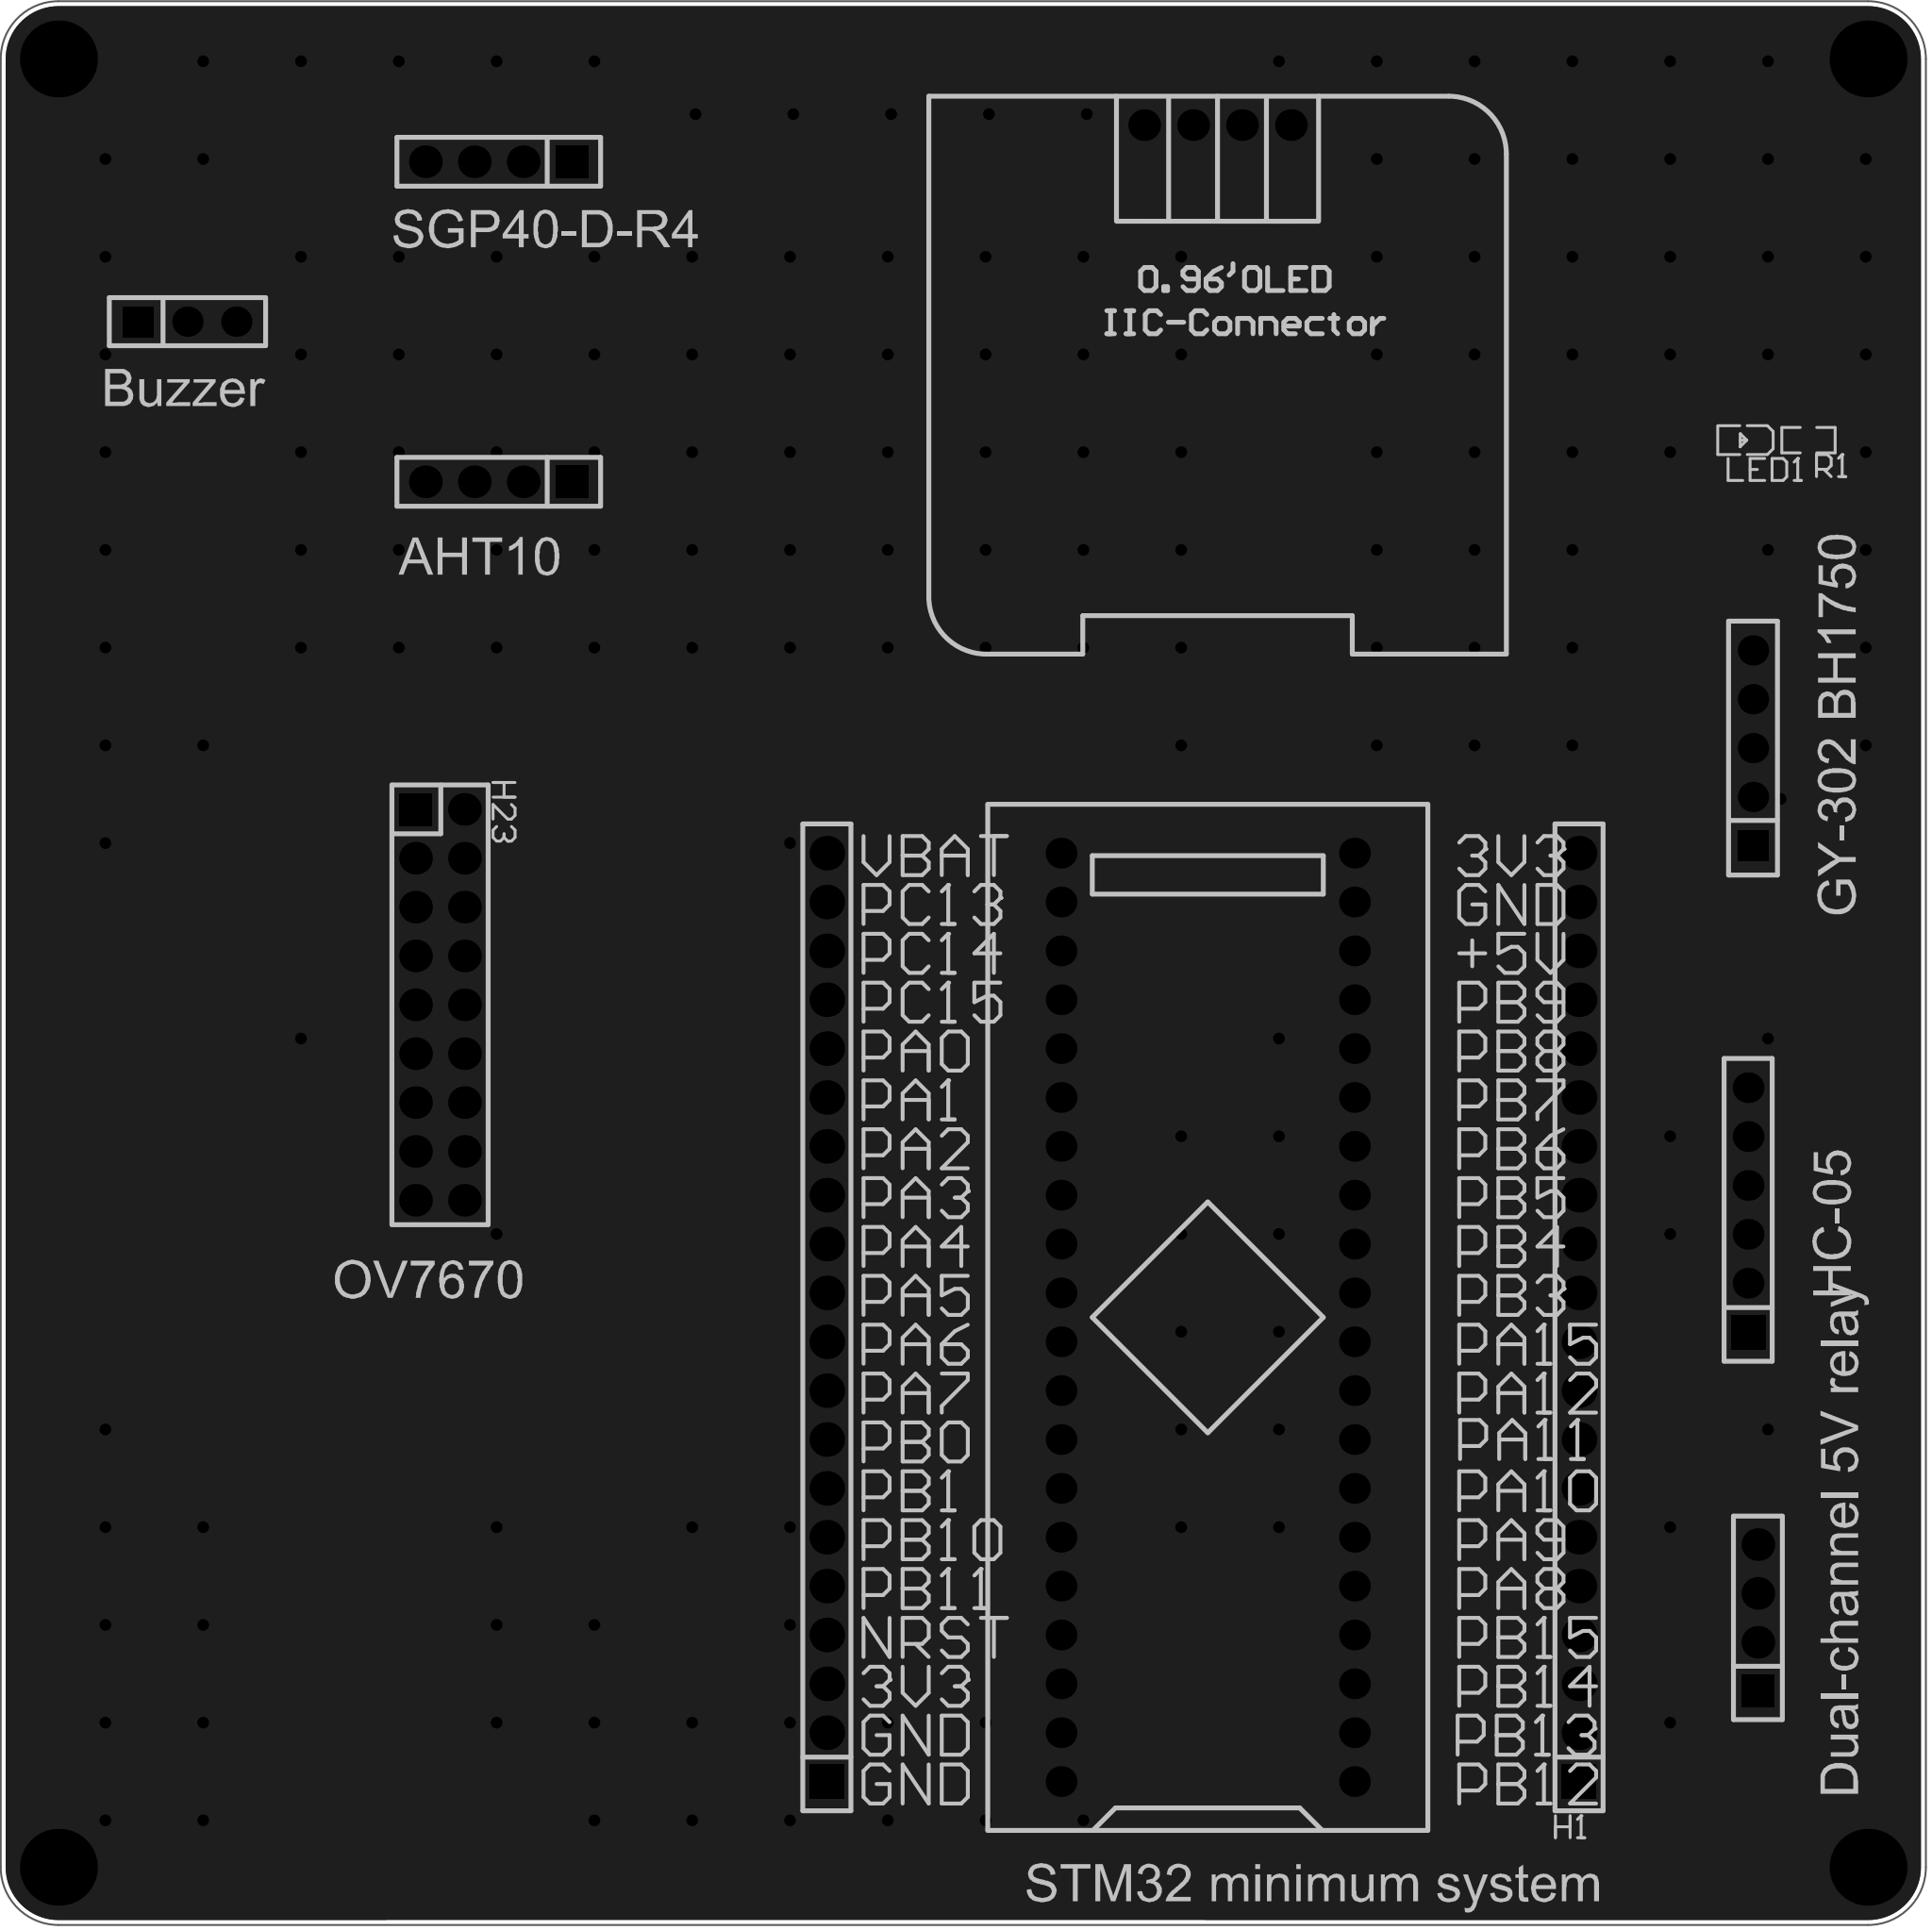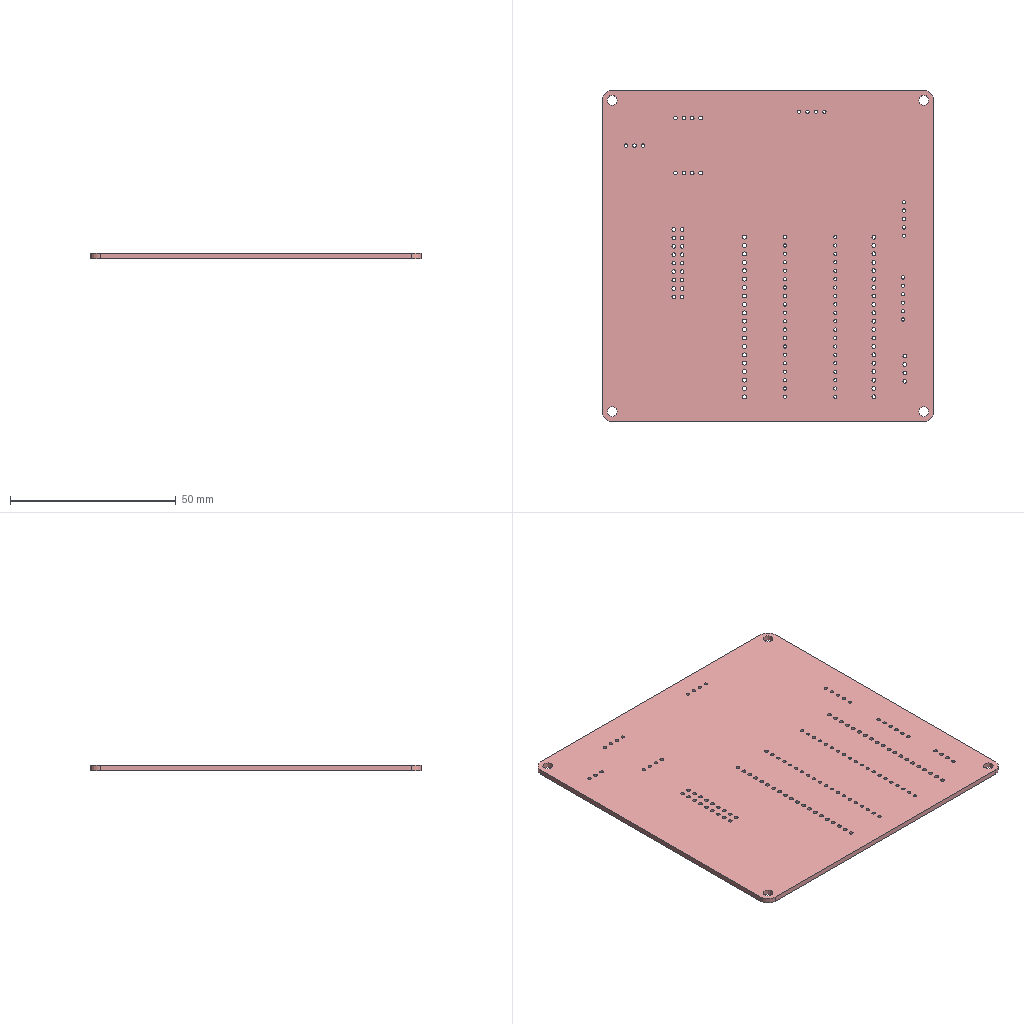Circuit board layout | Altium Designer | box 100 x 100 x 1.6 mm
Layer stack:
# Altium Designer layer stack of  (unit mm; dielectric type: 0 none, 1 core, 2 prepreg, 3 surface material)
index,name,kind,layer,copper_thickness_mm,dielectric_type,dielectric_thickness_mm,dielectric_material,dielectric_constant
0,Top Paste Mask Layer,other,,,,,,
1,Top Silkscreen Layer,other,,,,,,
2,Top Solder Mask Layer,dielectric,,,3,0.01,,3.3
3,Top Layer,copper,Top Layer,0.035,,,,
4,Dielectric1,dielectric,,,3,1.51,FR4,4.5
5,Bottom Layer,copper,Bottom Layer,0.035,,,,
6,Bottom Solder Mask Layer,dielectric,,,3,0.01,,3.3
7,Bottom Silkscreen Layer,other,,,,,,
8,Bottom Paste Mask Layer,other,,,,,,
# drill layer pairs: low layer,high layer
drill_pair,Top Layer,Bottom Layer
Part placement:
Designator,Comment,Layer,Footprint,Center-X(mm),Center-Y(mm),Rotation
U1,STM32F103C8T6-Card,TopLayer,CONN-TH_L53.3-W22.9_STM32F103C8T6-CARD,143.256,110.49,90
H23,,TopLayer,HDR-TH_18P-P2.54-V-M-R2-C9-S2.54,103.375,126.737,270
H19,,TopLayer,HDR-TH_4P-P2.54-V-F,106.426,153.924,180
OLED1,,TopLayer,0.96OLED_4P,143.764,172.466,0
H20,,TopLayer,HDR-TH_4P-P2.54-V-F,106.426,170.561,180
H21,,TopLayer,HDR-TH_5P-P2.54-V-F,171.577,140.081,90
H22,,TopLayer,HDR-TH_4P-P2.54-V-F,171.831,94.869,90
H1,,TopLayer,HDR-TH_20P-P2.54-V-F,162.539,110.49,90
H2,,TopLayer,HDR-TH_20P-P2.54-V-F,123.468,110.49,90
H25,,TopLayer,HDR-TH_3P-P2.54-V-F,90.256,162.248,0
LED1,,TopLayer,LED_0603,171.134,156.096,180
R1,510,TopLayer,R0603,174.458,156.088,0
H24,,TopLayer,HDR-TH_6P-P2.54-V-F,171.323,116.078,90
Pad and via stacks:
# Altium Designer via and pad stacks of  (unit mm). Each distinct definition once, with the count of objects using it.
# via: kind,start_layer,end_layer,hole_mm,diameter_mm,mode(0 simple;1 top-mid-bottom;2 full stack),diameter_per_layer,count,example_net
# pad: kind,layer,hole_mm,hole_type(0 round;1 square;2 slot),plating,top_size,top_shape(1 round;2 rect;3 octagon;9 rounded rect),mid_size,bottom_size,mode,footprint,size_per_layer,count,example
pad,Multi-Layer,3,0,plated,4x4,1,4x4,4x4,0,,,4,1
pad,Multi-Layer,1,0,plated,1.6x1.6,1,1.6x1.6,1.6x1.6,0,CONN-TH_L53.3-W22.9_STM32F103C8T6-CARD,,40,U1.1
pad,Multi-Layer,1.1,0,plated,1.7x1.7,2,1.7x1.7,1.7x1.7,0,HDR-TH_18P-P2.54-V-M-R2-C9-S2.54,,1,H23.1
pad,Multi-Layer,1.1,0,plated,1.7x1.7,1,1.7x1.7,1.7x1.7,0,HDR-TH_18P-P2.54-V-M-R2-C9-S2.54,,17,H23.2
pad,Multi-Layer,1.1,0,plated,1.7x1.7,2,1.7x1.7,1.7x1.7,0,HDR-TH_4P-P2.54-V-F,,3,H19.1
pad,Multi-Layer,1.1,0,plated,1.7x1.7,1,1.7x1.7,1.7x1.7,0,HDR-TH_4P-P2.54-V-F,,9,H19.2
pad,Multi-Layer,1,0,plated,1.65x1.65,1,1.65x1.65,1.65x1.65,0,0.96OLED_4P,,4,OLED1.4
pad,Multi-Layer,1.02,0,plated,1.575x1.575,1,1.575x1.575,1.575x1.575,0,HDR-TH_5P-P2.54-V-F,,4,H21.5
pad,Multi-Layer,1.02,0,plated,1.575x1.575,2,1.575x1.575,1.575x1.575,0,HDR-TH_5P-P2.54-V-F,,1,H21.1
pad,Multi-Layer,1.2,0,plated,1.8x1.8,2,1.8x1.8,1.8x1.8,0,HDR-TH_20P-P2.54-V-F,,2,H1.1
pad,Multi-Layer,1.2,0,plated,1.8x1.8,1,1.8x1.8,1.8x1.8,0,HDR-TH_20P-P2.54-V-F,,38,H1.2
pad,Multi-Layer,1.02,0,plated,1.575x1.575,1,1.575x1.575,1.575x1.575,0,HDR-TH_3P-P2.54-V-F,,2,H25.3
pad,Multi-Layer,1.02,0,plated,1.575x1.575,2,1.575x1.575,1.575x1.575,0,HDR-TH_3P-P2.54-V-F,,1,H25.1
pad,Multi-Layer,1.02,0,plated,1.6x1.6,1,1.6x1.6,1.6x1.6,0,HDR-TH_6P-P2.54-V-F,,5,H24.6
pad,Multi-Layer,1.02,0,plated,1.8x1.8,2,1.8x1.8,1.8x1.8,0,HDR-TH_6P-P2.54-V-F,,1,H24.1
pad,Top Layer,0,0,plated,0.8001x0.8001,2,0.8001x0.8001,0.8001x0.8001,0,LED_0603,,2,LED1.1
pad,Top Layer,0,0,plated,0.8065x0.864,2,0.8065x0.864,0.8065x0.864,0,R0603,,2,R1.2
via,Top Layer,Bottom Layer,0.3048,0.61,0,,161,GND
Copper pours:
name,layer,net,type(0 solid;1 hatched;2 none)
Bottom Layer-GND,Bottom Layer,GND,0
Top Layer-GND,Top Layer,GND,0